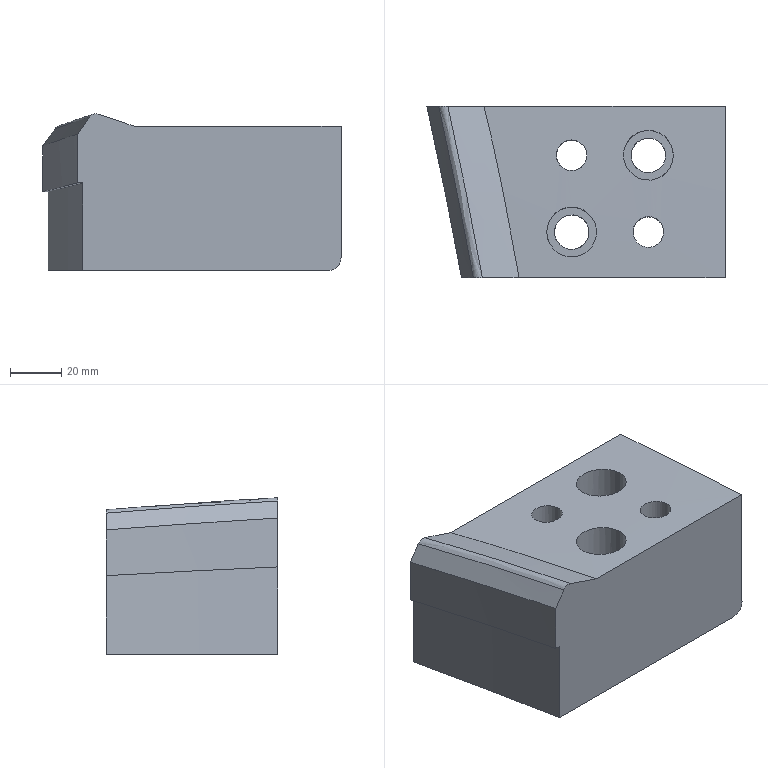Part | NX | features MAIN_BODY 2 | 1 solid | 22 faces | box 116.607 x 67 x 61.287 mm | volume 354263 mm3 | spline 9 | cylinder 7 | plane 6 | commonest cylinder face diameters 12 x2 13.5 x2 19.5 x2 10 x1
STEP:
#1=CARTESIAN_POINT('',(875.592,391.799,-36.703));
#2=VERTEX_POINT('',#1);
#3=CARTESIAN_POINT('',(875.621,399.722,-37.284));
#4=CARTESIAN_POINT('',(874.575,391.522,-36.682));
#5=CARTESIAN_POINT('',(879.631,384.982,-36.205));
#6=CARTESIAN_POINT('',(887.838,383.931,-36.131));
#7=CARTESIAN_POINT('',(894.382,388.999,-36.496));
#8=CARTESIAN_POINT('',(895.422,397.191,-37.099));
#9=CARTESIAN_POINT('',(890.383,403.727,-37.578));
#10=CARTESIAN_POINT('',(882.165,404.789,-37.656));
#11=CARTESIAN_POINT('',(875.621,399.722,-37.284));
#12=CARTESIAN_POINT('',(874.575,391.522,-36.682));
#13=CARTESIAN_POINT('',(879.631,384.982,-36.205));
#14=B_SPLINE_CURVE_WITH_KNOTS('',3,(#3,#4,#5,#6,#7,#8,#9,#10,#11,#12,#13),.UNSPECIFIED.,.T.,.F.,(1,1,1,1,1,1,1,1,1,1,1,1,1,1,1),(-0.02289,-0.01526,-0.00763,0.,0.00763,0.01526,0.02289,0.03052,0.03815,0.04578,0.05341,0.06104,0.06867,0.0763,0.08393),.UNSPECIFIED.);
#15=EDGE_CURVE('',#2,#2,#14,.T.);
#16=ORIENTED_EDGE('',*,*,#15,.F.);
#17=EDGE_LOOP('',(#16));
#18=FACE_BOUND('',#17,.T.);
#19=CARTESIAN_POINT('',(883.489,358.552,-34.446));
#20=VERTEX_POINT('',#19);
#21=CARTESIAN_POINT('',(879.261,361.,-34.597));
#22=CARTESIAN_POINT('',(883.325,357.92,-34.407));
#23=CARTESIAN_POINT('',(888.373,358.629,-34.45));
#24=CARTESIAN_POINT('',(891.432,362.685,-34.703));
#25=CARTESIAN_POINT('',(890.737,367.72,-35.026));
#26=CARTESIAN_POINT('',(886.676,370.794,-35.229));
#27=CARTESIAN_POINT('',(881.635,370.093,-35.183));
#28=CARTESIAN_POINT('',(878.567,366.035,-34.917));
#29=CARTESIAN_POINT('',(879.261,361.,-34.597));
#30=CARTESIAN_POINT('',(883.325,357.92,-34.407));
#31=CARTESIAN_POINT('',(888.373,358.629,-34.45));
#32=B_SPLINE_CURVE_WITH_KNOTS('',3,(#21,#22,#23,#24,#25,#26,#27,#28,#29,#30,#31),.UNSPECIFIED.,.T.,.F.,(1,1,1,1,1,1,1,1,1,1,1,1,1,1,1),(-0.01408,-0.009388,-0.004694,0.,0.004694,0.009388,0.01408,0.01878,0.02347,0.02816,0.03286,0.03755,0.04225,0.04694,0.05163),.UNSPECIFIED.);
#33=EDGE_CURVE('',#20,#20,#32,.T.);
#34=ORIENTED_EDGE('',*,*,#33,.F.);
#35=EDGE_LOOP('',(#34));
#36=FACE_BOUND('',#35,.T.);
#37=CARTESIAN_POINT('',(854.401,388.388,-36.453));
#38=VERTEX_POINT('',#37);
#39=CARTESIAN_POINT('',(849.844,390.159,-36.582));
#40=CARTESIAN_POINT('',(854.336,387.739,-36.405));
#41=CARTESIAN_POINT('',(859.216,389.217,-36.513));
#42=CARTESIAN_POINT('',(861.612,393.692,-36.842));
#43=CARTESIAN_POINT('',(860.154,398.56,-37.199));
#44=CARTESIAN_POINT('',(855.666,400.976,-37.376));
#45=CARTESIAN_POINT('',(850.791,399.506,-37.268));
#46=CARTESIAN_POINT('',(848.387,395.026,-36.939));
#47=CARTESIAN_POINT('',(849.844,390.159,-36.582));
#48=CARTESIAN_POINT('',(854.336,387.739,-36.405));
#49=CARTESIAN_POINT('',(859.216,389.217,-36.513));
#50=B_SPLINE_CURVE_WITH_KNOTS('',3,(#39,#40,#41,#42,#43,#44,#45,#46,#47,#48,#49),.UNSPECIFIED.,.T.,.F.,(1,1,1,1,1,1,1,1,1,1,1,1,1,1,1),(-0.01409,-0.009391,-0.004696,0.,0.004696,0.009391,0.01409,0.01878,0.02348,0.02817,0.03287,0.03756,0.04226,0.04696,0.05165),.UNSPECIFIED.);
#51=EDGE_CURVE('',#38,#38,#50,.T.);
#52=ORIENTED_EDGE('',*,*,#51,.F.);
#53=EDGE_LOOP('',(#52));
#54=FACE_BOUND('',#53,.T.);
#55=CARTESIAN_POINT('',(858.083,355.109,-34.235));
#56=VERTEX_POINT('',#55);
#57=CARTESIAN_POINT('',(850.147,354.7,-34.209));
#58=CARTESIAN_POINT('',(858.421,354.104,-34.174));
#59=CARTESIAN_POINT('',(864.664,359.534,-34.503));
#60=CARTESIAN_POINT('',(865.251,367.759,-35.026));
#61=CARTESIAN_POINT('',(859.849,374.018,-35.444));
#62=CARTESIAN_POINT('',(851.583,374.61,-35.485));
#63=CARTESIAN_POINT('',(845.343,369.198,-35.121));
#64=CARTESIAN_POINT('',(844.745,360.963,-34.592));
#65=CARTESIAN_POINT('',(850.147,354.7,-34.209));
#66=CARTESIAN_POINT('',(858.421,354.104,-34.174));
#67=CARTESIAN_POINT('',(864.664,359.534,-34.503));
#68=B_SPLINE_CURVE_WITH_KNOTS('',3,(#57,#58,#59,#60,#61,#62,#63,#64,#65,#66,#67),.UNSPECIFIED.,.T.,.F.,(1,1,1,1,1,1,1,1,1,1,1,1,1,1,1),(-0.02288,-0.01526,-0.007628,0.,0.007628,0.01526,0.02288,0.03051,0.03814,0.04577,0.05339,0.06102,0.06865,0.07628,0.0839),.UNSPECIFIED.);
#69=EDGE_CURVE('',#56,#56,#68,.T.);
#70=ORIENTED_EDGE('',*,*,#69,.F.);
#71=EDGE_LOOP('',(#70));
#72=FACE_BOUND('',#71,.T.);
#73=CARTESIAN_POINT('',(915.,346.533,-33.724));
#74=VERTEX_POINT('',#73);
#75=CARTESIAN_POINT('',(834.457,346.533,-33.724));
#76=VERTEX_POINT('',#75);
#77=CARTESIAN_POINT('',(873.245,346.533,-33.724));
#78=DIRECTION('',(-1.,0.000000011,-0.000000341));
#79=VECTOR('',#78,1000.);
#80=LINE('',#77,#79);
#81=EDGE_CURVE('',#74,#76,#80,.T.);
#82=ORIENTED_EDGE('',*,*,#81,.F.);
#83=CARTESIAN_POINT('',(915.,413.533,-38.297));
#84=VERTEX_POINT('',#83);
#85=CARTESIAN_POINT('',(915.,413.533,-38.297));
#86=CARTESIAN_POINT('',(915.,402.37,-37.478));
#87=CARTESIAN_POINT('',(915.,380.048,-35.784));
#88=CARTESIAN_POINT('',(915.,357.706,-34.385));
#89=CARTESIAN_POINT('',(915.,346.533,-33.724));
#90=B_SPLINE_CURVE_WITH_KNOTS('',3,(#85,#86,#87,#88,#89),.UNSPECIFIED.,.F.,.F.,(4,1,4),(0.271,0.3046,0.3382),.UNSPECIFIED.);
#91=EDGE_CURVE('',#84,#74,#90,.T.);
#92=ORIENTED_EDGE('',*,*,#91,.F.);
#93=CARTESIAN_POINT('',(820.678,413.533,-38.297));
#94=VERTEX_POINT('',#93);
#95=CARTESIAN_POINT('',(866.342,413.533,-38.297));
#96=DIRECTION('',(-1.,0.000000011,-0.000000341));
#97=VECTOR('',#96,1000.);
#98=LINE('',#95,#97);
#99=EDGE_CURVE('',#84,#94,#98,.T.);
#100=ORIENTED_EDGE('',*,*,#99,.T.);
#101=CARTESIAN_POINT('',(820.678,413.533,-38.297));
#102=CARTESIAN_POINT('',(822.089,408.009,-37.892));
#103=CARTESIAN_POINT('',(824.735,396.922,-37.08));
#104=CARTESIAN_POINT('',(829.299,374.584,-35.434));
#105=CARTESIAN_POINT('',(832.519,357.777,-34.389));
#106=CARTESIAN_POINT('',(834.457,346.533,-33.724));
#107=B_SPLINE_CURVE_WITH_KNOTS('',3,(#101,#102,#103,#104,#105,#106),.UNSPECIFIED.,.F.,.F.,(4,1,1,4),(0.,0.01714,0.03428,0.06856),.UNSPECIFIED.);
#108=EDGE_CURVE('',#94,#76,#107,.T.);
#109=ORIENTED_EDGE('',*,*,#108,.T.);
#110=EDGE_LOOP('',(#82,#92,#100,#109));
#111=FACE_BOUND('',#110,.T.);
#112=CARTESIAN_POINT('',(929.074,346.533,-33.724));
#113=CARTESIAN_POINT('',(833.62,346.533,-33.724));
#114=CARTESIAN_POINT('',(927.029,357.74,-34.387));
#115=CARTESIAN_POINT('',(831.575,357.74,-34.387));
#116=CARTESIAN_POINT('',(922.77,380.157,-35.792));
#117=CARTESIAN_POINT('',(827.316,380.157,-35.792));
#118=CARTESIAN_POINT('',(917.93,402.399,-37.48));
#119=CARTESIAN_POINT('',(822.476,402.399,-37.48));
#120=CARTESIAN_POINT('',(915.566,413.533,-38.297));
#121=CARTESIAN_POINT('',(820.112,413.533,-38.297));
#122=B_SPLINE_SURFACE_WITH_KNOTS('',3,1,((#112,#113),(#114,#115),(#116,#117),(#118,#119),(#120,#121)),.SURF_OF_LINEAR_EXTRUSION.,.F.,.F.,.F.,(4,1,4),(2,2),(-0.1003,0.757,1.614),(0.,1.),.UNSPECIFIED.);
#123=ADVANCED_FACE('',(#18,#36,#54,#72,#111),#122,.T.);
#124=CARTESIAN_POINT('',(798.461,413.533,-41.305));
#125=VERTEX_POINT('',#124);
#126=CARTESIAN_POINT('',(798.393,413.533,-41.305));
#127=VERTEX_POINT('',#126);
#128=CARTESIAN_POINT('',(871.04,413.533,-41.305));
#129=DIRECTION('',(-1.,0.000000011,-0.000000341));
#130=VECTOR('',#129,1000.);
#131=LINE('',#128,#130);
#132=EDGE_CURVE('',#125,#127,#131,.T.);
#133=ORIENTED_EDGE('',*,*,#132,.T.);
#134=CARTESIAN_POINT('',(804.549,384.498,-39.18));
#135=VERTEX_POINT('',#134);
#136=CARTESIAN_POINT('',(798.393,413.533,-41.305));
#137=CARTESIAN_POINT('',(800.448,403.855,-40.595));
#138=CARTESIAN_POINT('',(802.53,394.184,-39.872));
#139=CARTESIAN_POINT('',(804.549,384.498,-39.18));
#140=B_SPLINE_CURVE_WITH_KNOTS('',3,(#136,#137,#138,#139),.UNSPECIFIED.,.F.,.F.,(4,4),(0.,0.02976),.UNSPECIFIED.);
#141=EDGE_CURVE('',#127,#135,#140,.T.);
#142=ORIENTED_EDGE('',*,*,#141,.T.);
#143=CARTESIAN_POINT('',(798.461,413.533,-41.305));
#144=CARTESIAN_POINT('',(800.491,403.855,-40.595));
#145=CARTESIAN_POINT('',(802.531,394.18,-39.872));
#146=CARTESIAN_POINT('',(804.549,384.498,-39.18));
#147=B_SPLINE_CURVE_WITH_KNOTS('',3,(#143,#144,#145,#146),.UNSPECIFIED.,.F.,.F.,(4,4),(0.,0.02974),.UNSPECIFIED.);
#148=EDGE_CURVE('',#125,#135,#147,.T.);
#149=ORIENTED_EDGE('',*,*,#148,.F.);
#150=EDGE_LOOP('',(#133,#142,#149));
#151=FACE_BOUND('',#150,.T.);
#152=CARTESIAN_POINT('',(804.654,384.324,-39.167));
#153=CARTESIAN_POINT('',(804.586,384.324,-39.167));
#154=CARTESIAN_POINT('',(802.624,394.068,-39.863));
#155=CARTESIAN_POINT('',(802.556,394.068,-39.863));
#156=CARTESIAN_POINT('',(800.529,403.797,-40.591));
#157=CARTESIAN_POINT('',(800.461,403.797,-40.591));
#158=CARTESIAN_POINT('',(798.461,413.533,-41.305));
#159=CARTESIAN_POINT('',(798.393,413.533,-41.305));
#160=B_SPLINE_SURFACE_WITH_KNOTS('',3,1,((#152,#153),(#154,#155),(#156,#157),(#158,#159)),.SURF_OF_LINEAR_EXTRUSION.,.F.,.F.,.F.,(4,4),(2,2),(0.8703,1.62),(0.,1.),.PIECEWISE_BEZIER_KNOTS.);
#161=ADVANCED_FACE('',(#151),#160,.T.);
#162=CARTESIAN_POINT('',(885.,387.608,-90.));
#163=VERTEX_POINT('',#162);
#164=CARTESIAN_POINT('',(885.,394.358,-90.));
#165=DIRECTION('',(0.000000341,-0.00000017,-1.));
#166=DIRECTION('',(-0.000000011,-1.,0.00000017));
#167=AXIS2_PLACEMENT_3D('',#164,#165,#166);
#168=CIRCLE('',#167,6.75);
#169=EDGE_CURVE('',#163,#163,#168,.T.);
#170=ORIENTED_EDGE('',*,*,#169,.F.);
#171=EDGE_LOOP('',(#170));
#172=FACE_BOUND('',#171,.T.);
#173=CARTESIAN_POINT('',(885.,358.358,-90.));
#174=VERTEX_POINT('',#173);
#175=CARTESIAN_POINT('',(885.,364.358,-90.));
#176=DIRECTION('',(0.000000341,-0.00000017,-1.));
#177=DIRECTION('',(-0.000000011,-1.,0.00000017));
#178=AXIS2_PLACEMENT_3D('',#175,#176,#177);
#179=CIRCLE('',#178,6.);
#180=EDGE_CURVE('',#174,#174,#179,.T.);
#181=ORIENTED_EDGE('',*,*,#180,.F.);
#182=EDGE_LOOP('',(#181));
#183=FACE_BOUND('',#182,.T.);
#184=CARTESIAN_POINT('',(855.,357.608,-90.));
#185=VERTEX_POINT('',#184);
#186=CARTESIAN_POINT('',(855.,364.358,-90.));
#187=DIRECTION('',(0.000000341,-0.00000017,-1.));
#188=DIRECTION('',(-0.000000011,-1.,0.00000017));
#189=AXIS2_PLACEMENT_3D('',#186,#187,#188);
#190=CIRCLE('',#189,6.75);
#191=EDGE_CURVE('',#185,#185,#190,.T.);
#192=ORIENTED_EDGE('',*,*,#191,.F.);
#193=EDGE_LOOP('',(#192));
#194=FACE_BOUND('',#193,.T.);
#195=CARTESIAN_POINT('',(855.,388.358,-90.));
#196=VERTEX_POINT('',#195);
#197=CARTESIAN_POINT('',(855.,394.358,-90.));
#198=DIRECTION('',(0.000000341,-0.00000017,-1.));
#199=DIRECTION('',(-0.000000011,-1.,0.00000017));
#200=AXIS2_PLACEMENT_3D('',#197,#198,#199);
#201=CIRCLE('',#200,6.);
#202=EDGE_CURVE('',#196,#196,#201,.T.);
#203=ORIENTED_EDGE('',*,*,#202,.F.);
#204=EDGE_LOOP('',(#203));
#205=FACE_BOUND('',#204,.T.);
#206=CARTESIAN_POINT('',(910.,346.533,-90.));
#207=VERTEX_POINT('',#206);
#208=CARTESIAN_POINT('',(813.948,346.533,-90.));
#209=VERTEX_POINT('',#208);
#210=CARTESIAN_POINT('',(830.,346.533,-90.));
#211=DIRECTION('',(-1.,0.000000011,-0.000000341));
#212=VECTOR('',#211,1000.);
#213=LINE('',#210,#212);
#214=EDGE_CURVE('',#207,#209,#213,.T.);
#215=ORIENTED_EDGE('',*,*,#214,.T.);
#216=CARTESIAN_POINT('',(800.438,413.533,-90.));
#217=VERTEX_POINT('',#216);
#218=CARTESIAN_POINT('',(800.438,413.533,-90.));
#219=CARTESIAN_POINT('',(802.804,402.389,-90.));
#220=CARTESIAN_POINT('',(807.649,380.124,-90.));
#221=CARTESIAN_POINT('',(811.904,357.74,-90.));
#222=CARTESIAN_POINT('',(813.948,346.533,-90.));
#223=B_SPLINE_CURVE_WITH_KNOTS('',3,(#218,#219,#220,#221,#222),.UNSPECIFIED.,.F.,.F.,(4,1,4),(0.,0.03418,0.06835),.UNSPECIFIED.);
#224=EDGE_CURVE('',#217,#209,#223,.T.);
#225=ORIENTED_EDGE('',*,*,#224,.F.);
#226=CARTESIAN_POINT('',(910.,413.533,-90.));
#227=VERTEX_POINT('',#226);
#228=CARTESIAN_POINT('',(830.,413.533,-90.));
#229=DIRECTION('',(-1.,0.000000011,-0.000000341));
#230=VECTOR('',#229,1000.);
#231=LINE('',#228,#230);
#232=EDGE_CURVE('',#227,#217,#231,.T.);
#233=ORIENTED_EDGE('',*,*,#232,.F.);
#234=CARTESIAN_POINT('',(910.,413.533,-90.));
#235=DIRECTION('',(0.000000011,1.,-0.00000017));
#236=VECTOR('',#235,1000.);
#237=LINE('',#234,#236);
#238=EDGE_CURVE('',#207,#227,#237,.T.);
#239=ORIENTED_EDGE('',*,*,#238,.F.);
#240=EDGE_LOOP('',(#215,#225,#233,#239));
#241=FACE_BOUND('',#240,.T.);
#242=CARTESIAN_POINT('',(830.,1053.533,-90.));
#243=DIRECTION('',(0.000000341,-0.00000017,-1.));
#244=DIRECTION('',(0.000000011,1.,-0.00000017));
#245=AXIS2_PLACEMENT_3D('',#242,#243,#244);
#246=PLANE('',#245);
#247=ADVANCED_FACE('',(#172,#183,#194,#205,#241),#246,.T.);
#248=CARTESIAN_POINT('',(806.592,413.533,-33.58));
#249=VERTEX_POINT('',#248);
#250=CARTESIAN_POINT('',(806.592,413.533,-33.58));
#251=CARTESIAN_POINT('',(811.287,413.533,-35.152));
#252=CARTESIAN_POINT('',(815.982,413.533,-36.725));
#253=CARTESIAN_POINT('',(820.678,413.533,-38.297));
#254=B_SPLINE_CURVE_WITH_KNOTS('',3,(#250,#251,#252,#253),.UNSPECIFIED.,.F.,.F.,(4,4),(0.002341,0.0172),.UNSPECIFIED.);
#255=EDGE_CURVE('',#249,#94,#254,.T.);
#256=ORIENTED_EDGE('',*,*,#255,.T.);
#257=ORIENTED_EDGE('',*,*,#99,.F.);
#258=CARTESIAN_POINT('',(915.,413.533,-85.));
#259=VERTEX_POINT('',#258);
#260=CARTESIAN_POINT('',(915.,413.533,-90.));
#261=DIRECTION('',(0.000000341,-0.00000017,-1.));
#262=VECTOR('',#261,1000.);
#263=LINE('',#260,#262);
#264=EDGE_CURVE('',#259,#84,#263,.F.);
#265=ORIENTED_EDGE('',*,*,#264,.F.);
#266=CARTESIAN_POINT('',(910.,413.533,-85.));
#267=DIRECTION('',(-0.000000011,-1.,0.00000017));
#268=DIRECTION('',(-0.000000341,0.00000017,1.));
#269=AXIS2_PLACEMENT_3D('',#266,#267,#268);
#270=CIRCLE('',#269,5.);
#271=EDGE_CURVE('',#227,#259,#270,.T.);
#272=ORIENTED_EDGE('',*,*,#271,.F.);
#273=ORIENTED_EDGE('',*,*,#232,.T.);
#274=CARTESIAN_POINT('',(800.438,413.533,-59.211));
#275=VERTEX_POINT('',#274);
#276=CARTESIAN_POINT('',(800.438,413.533,-59.211));
#277=CARTESIAN_POINT('',(800.438,413.533,-69.474));
#278=CARTESIAN_POINT('',(800.438,413.533,-79.737));
#279=CARTESIAN_POINT('',(800.438,413.533,-90.));
#280=B_SPLINE_CURVE_WITH_KNOTS('',3,(#276,#277,#278,#279),.UNSPECIFIED.,.F.,.F.,(4,4),(0.,0.03079),.UNSPECIFIED.);
#281=EDGE_CURVE('',#275,#217,#280,.T.);
#282=ORIENTED_EDGE('',*,*,#281,.F.);
#283=CARTESIAN_POINT('',(798.393,413.533,-59.226));
#284=VERTEX_POINT('',#283);
#285=CARTESIAN_POINT('',(800.438,413.533,-59.211));
#286=CARTESIAN_POINT('',(799.756,413.533,-59.216));
#287=CARTESIAN_POINT('',(799.075,413.533,-59.221));
#288=CARTESIAN_POINT('',(798.393,413.533,-59.226));
#289=B_SPLINE_CURVE_WITH_KNOTS('',3,(#285,#286,#287,#288),.UNSPECIFIED.,.F.,.F.,(4,4),(0.003448,0.005492),.UNSPECIFIED.);
#290=EDGE_CURVE('',#275,#284,#289,.T.);
#291=ORIENTED_EDGE('',*,*,#290,.T.);
#292=CARTESIAN_POINT('',(798.393,413.533,-41.305));
#293=CARTESIAN_POINT('',(798.393,413.533,-47.279));
#294=CARTESIAN_POINT('',(798.393,413.533,-53.252));
#295=CARTESIAN_POINT('',(798.393,413.533,-59.226));
#296=B_SPLINE_CURVE_WITH_KNOTS('',3,(#292,#293,#294,#295),.UNSPECIFIED.,.F.,.F.,(4,4),(0.,0.01792),.UNSPECIFIED.);
#297=EDGE_CURVE('',#127,#284,#296,.T.);
#298=ORIENTED_EDGE('',*,*,#297,.F.);
#299=ORIENTED_EDGE('',*,*,#132,.F.);
#300=CARTESIAN_POINT('',(803.028,413.533,-34.762));
#301=VERTEX_POINT('',#300);
#302=CARTESIAN_POINT('',(803.028,413.533,-34.762));
#303=CARTESIAN_POINT('',(801.506,413.533,-36.943));
#304=CARTESIAN_POINT('',(799.983,413.533,-39.124));
#305=CARTESIAN_POINT('',(798.461,413.533,-41.305));
#306=B_SPLINE_CURVE_WITH_KNOTS('',3,(#302,#303,#304,#305),.UNSPECIFIED.,.F.,.F.,(4,4),(0.002349,0.01033),.UNSPECIFIED.);
#307=EDGE_CURVE('',#301,#125,#306,.T.);
#308=ORIENTED_EDGE('',*,*,#307,.F.);
#309=CARTESIAN_POINT('',(806.592,413.533,-33.58));
#310=CARTESIAN_POINT('',(805.308,413.533,-33.15));
#311=CARTESIAN_POINT('',(803.802,413.533,-33.652));
#312=CARTESIAN_POINT('',(803.028,413.533,-34.762));
#313=B_SPLINE_CURVE_WITH_KNOTS('',3,(#309,#310,#311,#312),.UNSPECIFIED.,.F.,.F.,(4,4),(0.,0.004002),.UNSPECIFIED.);
#314=EDGE_CURVE('',#249,#301,#313,.T.);
#315=ORIENTED_EDGE('',*,*,#314,.F.);
#316=EDGE_LOOP('',(#256,#257,#265,#272,#273,#282,#291,#298,#299,#308,#315));
#317=FACE_BOUND('',#316,.T.);
#318=CARTESIAN_POINT('',(890.,413.533,-90.));
#319=DIRECTION('',(0.000000011,1.,-0.00000017));
#320=DIRECTION('',(-0.000000341,0.00000017,1.));
#321=AXIS2_PLACEMENT_3D('',#318,#319,#320);
#322=PLANE('',#321);
#323=ADVANCED_FACE('',(#317),#322,.T.);
#324=ORIENTED_EDGE('',*,*,#141,.F.);
#325=ORIENTED_EDGE('',*,*,#297,.T.);
#326=CARTESIAN_POINT('',(811.915,346.533,-55.81));
#327=VERTEX_POINT('',#326);
#328=CARTESIAN_POINT('',(798.393,413.533,-59.226));
#329=CARTESIAN_POINT('',(800.759,402.391,-58.614));
#330=CARTESIAN_POINT('',(805.603,380.131,-57.36));
#331=CARTESIAN_POINT('',(809.87,357.743,-56.321));
#332=CARTESIAN_POINT('',(811.915,346.533,-55.81));
#333=B_SPLINE_CURVE_WITH_KNOTS('',3,(#328,#329,#330,#331,#332),.UNSPECIFIED.,.F.,.F.,(4,1,4),(0.,0.03422,0.06844),.UNSPECIFIED.);
#334=EDGE_CURVE('',#284,#327,#333,.T.);
#335=ORIENTED_EDGE('',*,*,#334,.T.);
#336=CARTESIAN_POINT('',(811.915,346.533,-36.73));
#337=VERTEX_POINT('',#336);
#338=CARTESIAN_POINT('',(811.915,346.533,-36.73));
#339=CARTESIAN_POINT('',(811.915,346.533,-43.09));
#340=CARTESIAN_POINT('',(811.915,346.533,-49.45));
#341=CARTESIAN_POINT('',(811.915,346.533,-55.81));
#342=B_SPLINE_CURVE_WITH_KNOTS('',3,(#338,#339,#340,#341),.UNSPECIFIED.,.F.,.F.,(4,4),(0.,0.01908),.UNSPECIFIED.);
#343=EDGE_CURVE('',#337,#327,#342,.T.);
#344=ORIENTED_EDGE('',*,*,#343,.F.);
#345=CARTESIAN_POINT('',(810.326,355.197,-37.246));
#346=VERTEX_POINT('',#345);
#347=CARTESIAN_POINT('',(810.326,355.197,-37.246));
#348=CARTESIAN_POINT('',(810.863,352.311,-37.07));
#349=CARTESIAN_POINT('',(811.388,349.422,-36.9));
#350=CARTESIAN_POINT('',(811.915,346.533,-36.73));
#351=B_SPLINE_CURVE_WITH_KNOTS('',3,(#347,#348,#349,#350),.UNSPECIFIED.,.F.,.F.,(4,4),(0.05968,0.06851),.UNSPECIFIED.);
#352=EDGE_CURVE('',#346,#337,#351,.T.);
#353=ORIENTED_EDGE('',*,*,#352,.F.);
#354=CARTESIAN_POINT('',(804.549,384.498,-39.18));
#355=CARTESIAN_POINT('',(806.58,374.756,-38.484));
#356=CARTESIAN_POINT('',(808.504,364.988,-37.841));
#357=CARTESIAN_POINT('',(810.326,355.197,-37.246));
#358=B_SPLINE_CURVE_WITH_KNOTS('',3,(#354,#355,#356,#357),.UNSPECIFIED.,.F.,.F.,(4,4),(0.02976,0.05969),.UNSPECIFIED.);
#359=EDGE_CURVE('',#135,#346,#358,.T.);
#360=ORIENTED_EDGE('',*,*,#359,.F.);
#361=EDGE_LOOP('',(#324,#325,#335,#344,#353,#360));
#362=FACE_BOUND('',#361,.T.);
#363=CARTESIAN_POINT('',(811.989,346.129,-55.901));
#364=CARTESIAN_POINT('',(811.989,346.129,-36.706));
#365=CARTESIAN_POINT('',(809.919,357.478,-56.572));
#366=CARTESIAN_POINT('',(809.919,357.478,-37.376));
#367=CARTESIAN_POINT('',(805.606,380.136,-57.992));
#368=CARTESIAN_POINT('',(805.606,380.136,-38.797));
#369=CARTESIAN_POINT('',(800.702,402.659,-59.703));
#370=CARTESIAN_POINT('',(800.702,402.659,-40.507));
#371=CARTESIAN_POINT('',(798.308,413.934,-60.53));
#372=CARTESIAN_POINT('',(798.308,413.934,-41.335));
#373=B_SPLINE_SURFACE_WITH_KNOTS('',3,1,((#363,#364),(#365,#366),(#367,#368),(#369,#370),(#371,#372)),.SURF_OF_LINEAR_EXTRUSION.,.F.,.F.,.F.,(4,1,4),(2,2),(-0.1061,0.7621,1.63),(0.,1.),.UNSPECIFIED.);
#374=ADVANCED_FACE('',(#362),#373,.F.);
#375=ORIENTED_EDGE('',*,*,#264,.T.);
#376=ORIENTED_EDGE('',*,*,#91,.T.);
#377=CARTESIAN_POINT('',(915.,346.533,-85.));
#378=VERTEX_POINT('',#377);
#379=CARTESIAN_POINT('',(915.,346.533,-90.));
#380=DIRECTION('',(0.000000341,-0.00000017,-1.));
#381=VECTOR('',#380,1000.);
#382=LINE('',#379,#381);
#383=EDGE_CURVE('',#378,#74,#382,.F.);
#384=ORIENTED_EDGE('',*,*,#383,.F.);
#385=CARTESIAN_POINT('',(915.,346.533,-85.));
#386=DIRECTION('',(-0.000000011,-1.,0.00000017));
#387=VECTOR('',#386,1000.);
#388=LINE('',#385,#387);
#389=EDGE_CURVE('',#259,#378,#388,.T.);
#390=ORIENTED_EDGE('',*,*,#389,.F.);
#391=EDGE_LOOP('',(#375,#376,#384,#390));
#392=FACE_BOUND('',#391,.T.);
#393=CARTESIAN_POINT('',(915.,734.25,-90.));
#394=DIRECTION('',(1.,-0.000000011,0.000000341));
#395=DIRECTION('',(0.000000341,-0.00000017,-1.));
#396=AXIS2_PLACEMENT_3D('',#393,#394,#395);
#397=PLANE('',#396);
#398=ADVANCED_FACE('',(#392),#397,.T.);
#399=ORIENTED_EDGE('',*,*,#352,.T.);
#400=CARTESIAN_POINT('',(811.931,346.533,-36.73));
#401=VERTEX_POINT('',#400);
#402=CARTESIAN_POINT('',(875.23,346.533,-36.73));
#403=DIRECTION('',(-1.,0.000000011,-0.000000341));
#404=VECTOR('',#403,1000.);
#405=LINE('',#402,#404);
#406=EDGE_CURVE('',#401,#337,#405,.T.);
#407=ORIENTED_EDGE('',*,*,#406,.F.);
#408=CARTESIAN_POINT('',(810.326,355.197,-37.246));
#409=CARTESIAN_POINT('',(810.863,352.31,-37.07));
#410=CARTESIAN_POINT('',(811.397,349.421,-36.9));
#411=CARTESIAN_POINT('',(811.931,346.533,-36.73));
#412=B_SPLINE_CURVE_WITH_KNOTS('',3,(#408,#409,#410,#411),.UNSPECIFIED.,.F.,.F.,(4,4),(0.05967,0.0685),.UNSPECIFIED.);
#413=EDGE_CURVE('',#346,#401,#412,.T.);
#414=ORIENTED_EDGE('',*,*,#413,.F.);
#415=EDGE_LOOP('',(#399,#407,#414));
#416=FACE_BOUND('',#415,.T.);
#417=CARTESIAN_POINT('',(811.931,346.533,-36.73));
#418=CARTESIAN_POINT('',(811.915,346.533,-36.73));
#419=CARTESIAN_POINT('',(811.401,349.439,-36.901));
#420=CARTESIAN_POINT('',(811.385,349.439,-36.901));
#421=CARTESIAN_POINT('',(810.872,352.345,-37.072));
#422=CARTESIAN_POINT('',(810.857,352.345,-37.072));
#423=CARTESIAN_POINT('',(810.332,355.249,-37.249));
#424=CARTESIAN_POINT('',(810.316,355.249,-37.249));
#425=B_SPLINE_SURFACE_WITH_KNOTS('',3,1,((#417,#418),(#419,#420),(#421,#422),(#423,#424)),.SURF_OF_LINEAR_EXTRUSION.,.F.,.F.,.F.,(4,4),(2,2),(-0.09577,0.1265),(0.,1.),.PIECEWISE_BEZIER_KNOTS.);
#426=ADVANCED_FACE('',(#416),#425,.T.);
#427=CARTESIAN_POINT('',(816.542,346.533,-30.039));
#428=VERTEX_POINT('',#427);
#429=CARTESIAN_POINT('',(811.931,346.533,-36.73));
#430=CARTESIAN_POINT('',(813.468,346.533,-34.5));
#431=CARTESIAN_POINT('',(815.005,346.533,-32.27));
#432=CARTESIAN_POINT('',(816.542,346.533,-30.039));
#433=B_SPLINE_CURVE_WITH_KNOTS('',3,(#429,#430,#431,#432),.UNSPECIFIED.,.F.,.F.,(4,4),(0.00002698,0.008152),.UNSPECIFIED.);
#434=EDGE_CURVE('',#401,#428,#433,.T.);
#435=ORIENTED_EDGE('',*,*,#434,.F.);
#436=ORIENTED_EDGE('',*,*,#406,.T.);
#437=ORIENTED_EDGE('',*,*,#343,.T.);
#438=CARTESIAN_POINT('',(813.948,346.533,-55.8));
#439=VERTEX_POINT('',#438);
#440=CARTESIAN_POINT('',(811.915,346.533,-55.81));
#441=CARTESIAN_POINT('',(812.593,346.533,-55.807));
#442=CARTESIAN_POINT('',(813.271,346.533,-55.803));
#443=CARTESIAN_POINT('',(813.948,346.533,-55.8));
#444=B_SPLINE_CURVE_WITH_KNOTS('',3,(#440,#441,#442,#443),.UNSPECIFIED.,.F.,.F.,(4,4),(0.001632,0.003665),.UNSPECIFIED.);
#445=EDGE_CURVE('',#327,#439,#444,.T.);
#446=ORIENTED_EDGE('',*,*,#445,.T.);
#447=CARTESIAN_POINT('',(813.948,346.533,-55.8));
#448=CARTESIAN_POINT('',(813.948,346.533,-67.2));
#449=CARTESIAN_POINT('',(813.948,346.533,-78.6));
#450=CARTESIAN_POINT('',(813.948,346.533,-90.));
#451=B_SPLINE_CURVE_WITH_KNOTS('',3,(#447,#448,#449,#450),.UNSPECIFIED.,.F.,.F.,(4,4),(0.,0.0342),.UNSPECIFIED.);
#452=EDGE_CURVE('',#439,#209,#451,.T.);
#453=ORIENTED_EDGE('',*,*,#452,.T.);
#454=ORIENTED_EDGE('',*,*,#214,.F.);
#455=CARTESIAN_POINT('',(910.,346.533,-85.));
#456=DIRECTION('',(-0.000000011,-1.,0.00000017));
#457=DIRECTION('',(-0.000000341,0.00000017,1.));
#458=AXIS2_PLACEMENT_3D('',#455,#456,#457);
#459=CIRCLE('',#458,5.);
#460=EDGE_CURVE('',#378,#207,#459,.F.);
#461=ORIENTED_EDGE('',*,*,#460,.F.);
#462=ORIENTED_EDGE('',*,*,#383,.T.);
#463=ORIENTED_EDGE('',*,*,#81,.T.);
#464=CARTESIAN_POINT('',(820.074,346.533,-28.867));
#465=VERTEX_POINT('',#464);
#466=CARTESIAN_POINT('',(820.074,346.533,-28.867));
#467=CARTESIAN_POINT('',(824.868,346.533,-30.486));
#468=CARTESIAN_POINT('',(829.662,346.533,-32.105));
#469=CARTESIAN_POINT('',(834.457,346.533,-33.724));
#470=B_SPLINE_CURVE_WITH_KNOTS('',3,(#466,#467,#468,#469),.UNSPECIFIED.,.F.,.F.,(4,4),(0.002332,0.01751),.UNSPECIFIED.);
#471=EDGE_CURVE('',#465,#76,#470,.T.);
#472=ORIENTED_EDGE('',*,*,#471,.F.);
#473=CARTESIAN_POINT('',(816.542,346.533,-30.039));
#474=CARTESIAN_POINT('',(817.304,346.533,-28.933));
#475=CARTESIAN_POINT('',(818.801,346.533,-28.437));
#476=CARTESIAN_POINT('',(820.074,346.533,-28.867));
#477=B_SPLINE_CURVE_WITH_KNOTS('',3,(#473,#474,#475,#476),.UNSPECIFIED.,.F.,.F.,(4,4),(0.,0.003971),.UNSPECIFIED.);
#478=EDGE_CURVE('',#428,#465,#477,.T.);
#479=ORIENTED_EDGE('',*,*,#478,.F.);
#480=EDGE_LOOP('',(#435,#436,#437,#446,#453,#454,#461,#462,#463,#472,#479));
#481=FACE_BOUND('',#480,.T.);
#482=CARTESIAN_POINT('',(890.,346.533,-90.));
#483=DIRECTION('',(0.000000011,1.,-0.00000017));
#484=DIRECTION('',(-0.000000341,0.00000017,1.));
#485=AXIS2_PLACEMENT_3D('',#482,#483,#484);
#486=PLANE('',#485);
#487=ADVANCED_FACE('',(#481),#486,.F.);
#488=CARTESIAN_POINT('',(894.75,394.358,-80.));
#489=VERTEX_POINT('',#488);
#490=CARTESIAN_POINT('',(885.,394.358,-80.));
#491=DIRECTION('',(-0.000000341,0.00000017,1.));
#492=DIRECTION('',(1.,0.,0.000000341));
#493=AXIS2_PLACEMENT_3D('',#490,#491,#492);
#494=CIRCLE('',#493,9.75);
#495=EDGE_CURVE('',#489,#489,#494,.F.);
#496=ORIENTED_EDGE('',*,*,#495,.T.);
#497=EDGE_LOOP('',(#496));
#498=FACE_BOUND('',#497,.T.);
#499=ORIENTED_EDGE('',*,*,#15,.T.);
#500=EDGE_LOOP('',(#499));
#501=FACE_BOUND('',#500,.T.);
#502=CARTESIAN_POINT('',(885.,394.358,-70.));
#503=DIRECTION('',(-0.000000341,0.00000017,1.));
#504=DIRECTION('',(-0.000000011,-1.,0.00000017));
#505=AXIS2_PLACEMENT_3D('',#502,#503,#504);
#506=CYLINDRICAL_SURFACE('',#505,9.75);
#507=ADVANCED_FACE('',(#498,#501),#506,.F.);
#508=CARTESIAN_POINT('',(891.75,394.358,-80.));
#509=VERTEX_POINT('',#508);
#510=CARTESIAN_POINT('',(885.,394.358,-80.));
#511=DIRECTION('',(-0.000000341,0.00000017,1.));
#512=DIRECTION('',(1.,0.,0.000000341));
#513=AXIS2_PLACEMENT_3D('',#510,#511,#512);
#514=CIRCLE('',#513,6.75);
#515=EDGE_CURVE('',#509,#509,#514,.F.);
#516=ORIENTED_EDGE('',*,*,#515,.F.);
#517=EDGE_LOOP('',(#516));
#518=FACE_BOUND('',#517,.T.);
#519=ORIENTED_EDGE('',*,*,#169,.T.);
#520=EDGE_LOOP('',(#519));
#521=FACE_BOUND('',#520,.T.);
#522=CARTESIAN_POINT('',(885.,394.358,-90.));
#523=DIRECTION('',(-0.000000341,0.00000017,1.));
#524=DIRECTION('',(-0.000000011,-1.,0.00000017));
#525=AXIS2_PLACEMENT_3D('',#522,#523,#524);
#526=CYLINDRICAL_SURFACE('',#525,6.75);
#527=ADVANCED_FACE('',(#518,#521),#526,.F.);
#528=ORIENTED_EDGE('',*,*,#515,.T.);
#529=EDGE_LOOP('',(#528));
#530=FACE_BOUND('',#529,.T.);
#531=ORIENTED_EDGE('',*,*,#495,.F.);
#532=EDGE_LOOP('',(#531));
#533=FACE_BOUND('',#532,.T.);
#534=CARTESIAN_POINT('',(885.,394.358,-80.));
#535=DIRECTION('',(0.000000341,-0.00000017,-1.));
#536=DIRECTION('',(0.000000011,1.,-0.00000017));
#537=AXIS2_PLACEMENT_3D('',#534,#535,#536);
#538=PLANE('',#537);
#539=ADVANCED_FACE('',(#530,#533),#538,.F.);
#540=ORIENTED_EDGE('',*,*,#180,.T.);
#541=EDGE_LOOP('',(#540));
#542=FACE_BOUND('',#541,.T.);
#543=ORIENTED_EDGE('',*,*,#33,.T.);
#544=EDGE_LOOP('',(#543));
#545=FACE_BOUND('',#544,.T.);
#546=CARTESIAN_POINT('',(885.,364.358,-90.));
#547=DIRECTION('',(-0.000000341,0.00000017,1.));
#548=DIRECTION('',(-0.000000011,-1.,0.00000017));
#549=AXIS2_PLACEMENT_3D('',#546,#547,#548);
#550=CYLINDRICAL_SURFACE('',#549,6.);
#551=ADVANCED_FACE('',(#542,#545),#550,.F.);
#552=CARTESIAN_POINT('',(864.75,364.358,-80.));
#553=VERTEX_POINT('',#552);
#554=CARTESIAN_POINT('',(855.,364.358,-80.));
#555=DIRECTION('',(-0.000000341,0.00000017,1.));
#556=DIRECTION('',(1.,0.,0.000000341));
#557=AXIS2_PLACEMENT_3D('',#554,#555,#556);
#558=CIRCLE('',#557,9.75);
#559=EDGE_CURVE('',#553,#553,#558,.F.);
#560=ORIENTED_EDGE('',*,*,#559,.T.);
#561=EDGE_LOOP('',(#560));
#562=FACE_BOUND('',#561,.T.);
#563=ORIENTED_EDGE('',*,*,#69,.T.);
#564=EDGE_LOOP('',(#563));
#565=FACE_BOUND('',#564,.T.);
#566=CARTESIAN_POINT('',(855.,364.358,-70.));
#567=DIRECTION('',(-0.000000341,0.00000017,1.));
#568=DIRECTION('',(-0.000000011,-1.,0.00000017));
#569=AXIS2_PLACEMENT_3D('',#566,#567,#568);
#570=CYLINDRICAL_SURFACE('',#569,9.75);
#571=ADVANCED_FACE('',(#562,#565),#570,.F.);
#572=CARTESIAN_POINT('',(861.75,364.358,-80.));
#573=VERTEX_POINT('',#572);
#574=CARTESIAN_POINT('',(855.,364.358,-80.));
#575=DIRECTION('',(-0.000000341,0.00000017,1.));
#576=DIRECTION('',(1.,0.,0.000000341));
#577=AXIS2_PLACEMENT_3D('',#574,#575,#576);
#578=CIRCLE('',#577,6.75);
#579=EDGE_CURVE('',#573,#573,#578,.F.);
#580=ORIENTED_EDGE('',*,*,#579,.F.);
#581=EDGE_LOOP('',(#580));
#582=FACE_BOUND('',#581,.T.);
#583=ORIENTED_EDGE('',*,*,#191,.T.);
#584=EDGE_LOOP('',(#583));
#585=FACE_BOUND('',#584,.T.);
#586=CARTESIAN_POINT('',(855.,364.358,-90.));
#587=DIRECTION('',(-0.000000341,0.00000017,1.));
#588=DIRECTION('',(-0.000000011,-1.,0.00000017));
#589=AXIS2_PLACEMENT_3D('',#586,#587,#588);
#590=CYLINDRICAL_SURFACE('',#589,6.75);
#591=ADVANCED_FACE('',(#582,#585),#590,.F.);
#592=ORIENTED_EDGE('',*,*,#579,.T.);
#593=EDGE_LOOP('',(#592));
#594=FACE_BOUND('',#593,.T.);
#595=ORIENTED_EDGE('',*,*,#559,.F.);
#596=EDGE_LOOP('',(#595));
#597=FACE_BOUND('',#596,.T.);
#598=CARTESIAN_POINT('',(855.,364.358,-80.));
#599=DIRECTION('',(0.000000341,-0.00000017,-1.));
#600=DIRECTION('',(0.000000011,1.,-0.00000017));
#601=AXIS2_PLACEMENT_3D('',#598,#599,#600);
#602=PLANE('',#601);
#603=ADVANCED_FACE('',(#594,#597),#602,.F.);
#604=ORIENTED_EDGE('',*,*,#202,.T.);
#605=EDGE_LOOP('',(#604));
#606=FACE_BOUND('',#605,.T.);
#607=ORIENTED_EDGE('',*,*,#51,.T.);
#608=EDGE_LOOP('',(#607));
#609=FACE_BOUND('',#608,.T.);
#610=CARTESIAN_POINT('',(855.,394.358,-90.));
#611=DIRECTION('',(-0.000000341,0.00000017,1.));
#612=DIRECTION('',(-0.000000011,-1.,0.00000017));
#613=AXIS2_PLACEMENT_3D('',#610,#611,#612);
#614=CYLINDRICAL_SURFACE('',#613,6.);
#615=ADVANCED_FACE('',(#606,#609),#614,.F.);
#616=ORIENTED_EDGE('',*,*,#290,.F.);
#617=CARTESIAN_POINT('',(800.438,413.533,-59.211));
#618=CARTESIAN_POINT('',(802.804,402.391,-58.6));
#619=CARTESIAN_POINT('',(807.647,380.132,-57.347));
#620=CARTESIAN_POINT('',(811.903,357.742,-56.311));
#621=CARTESIAN_POINT('',(813.948,346.533,-55.8));
#622=B_SPLINE_CURVE_WITH_KNOTS('',3,(#617,#618,#619,#620,#621),.UNSPECIFIED.,.F.,.F.,(4,1,4),(0.,0.03422,0.06844),.UNSPECIFIED.);
#623=EDGE_CURVE('',#275,#439,#622,.T.);
#624=ORIENTED_EDGE('',*,*,#623,.T.);
#625=ORIENTED_EDGE('',*,*,#445,.F.);
#626=ORIENTED_EDGE('',*,*,#334,.F.);
#627=EDGE_LOOP('',(#616,#624,#625,#626));
#628=FACE_BOUND('',#627,.T.);
#629=CARTESIAN_POINT('',(798.321,413.758,-59.238));
#630=CARTESIAN_POINT('',(798.35,413.533,-59.226));
#631=CARTESIAN_POINT('',(798.38,413.307,-59.214));
#632=CARTESIAN_POINT('',(798.409,413.082,-59.201));
#633=CARTESIAN_POINT('',(799.863,401.922,-58.595));
#634=CARTESIAN_POINT('',(801.338,390.768,-57.973));
#635=CARTESIAN_POINT('',(804.163,368.465,-56.841));
#636=CARTESIAN_POINT('',(805.488,357.305,-56.325));
#637=CARTESIAN_POINT('',(806.819,346.12,-55.819));
#638=CARTESIAN_POINT('',(806.846,345.897,-55.809));
#639=CARTESIAN_POINT('',(806.872,345.673,-55.799));
#640=CARTESIAN_POINT('',(806.899,345.449,-55.789));
#641=CARTESIAN_POINT('',(805.432,414.684,-59.238));
#642=CARTESIAN_POINT('',(805.461,414.459,-59.226));
#643=CARTESIAN_POINT('',(805.49,414.234,-59.214));
#644=CARTESIAN_POINT('',(805.52,414.008,-59.201));
#645=CARTESIAN_POINT('',(806.973,402.853,-58.596));
#646=CARTESIAN_POINT('',(808.449,391.697,-57.973));
#647=CARTESIAN_POINT('',(811.281,369.338,-56.841));
#648=CARTESIAN_POINT('',(812.61,358.14,-56.325));
#649=CARTESIAN_POINT('',(813.939,346.968,-55.819));
#650=CARTESIAN_POINT('',(813.966,346.744,-55.809));
#651=CARTESIAN_POINT('',(813.993,346.521,-55.799));
#652=CARTESIAN_POINT('',(814.019,346.297,-55.789));
#653=B_SPLINE_SURFACE_WITH_KNOTS('',1,3,((#629,#630,#631,#632,#633,#634,#635,#636,#637,#638,#639,#640),(#641,#642,#643,#644,#645,#646,#647,#648,#649,#650,#651,#652)),.RULED_SURF.,.F.,.F.,.F.,(2,2),(4,3,2,3,4),(0.1511,0.8682),(-0.0101,0.,0.5,1.,1.01),.UNSPECIFIED.);
#654=ADVANCED_FACE('',(#628),#653,.T.);
#655=ORIENTED_EDGE('',*,*,#623,.F.);
#656=ORIENTED_EDGE('',*,*,#281,.T.);
#657=ORIENTED_EDGE('',*,*,#224,.T.);
#658=ORIENTED_EDGE('',*,*,#452,.F.);
#659=EDGE_LOOP('',(#655,#656,#657,#658));
#660=FACE_BOUND('',#659,.T.);
#661=CARTESIAN_POINT('',(814.022,346.129,-90.188));
#662=CARTESIAN_POINT('',(814.022,346.129,-54.409));
#663=CARTESIAN_POINT('',(811.953,357.468,-90.858));
#664=CARTESIAN_POINT('',(811.953,357.468,-55.079));
#665=CARTESIAN_POINT('',(807.644,380.165,-92.272));
#666=CARTESIAN_POINT('',(807.644,380.165,-56.493));
#667=CARTESIAN_POINT('',(802.745,402.669,-93.981));
#668=CARTESIAN_POINT('',(802.745,402.669,-58.202));
#669=CARTESIAN_POINT('',(800.353,413.933,-94.808));
#670=CARTESIAN_POINT('',(800.353,413.933,-59.029));
#671=B_SPLINE_SURFACE_WITH_KNOTS('',3,1,((#661,#662),(#663,#664),(#665,#666),(#667,#668),(#669,#670)),.SURF_OF_LINEAR_EXTRUSION.,.F.,.F.,.F.,(4,1,4),(2,2),(-0.1152,0.7522,1.62),(0.,1.),.UNSPECIFIED.);
#672=ADVANCED_FACE('',(#660),#671,.F.);
#673=ORIENTED_EDGE('',*,*,#271,.T.);
#674=ORIENTED_EDGE('',*,*,#389,.T.);
#675=ORIENTED_EDGE('',*,*,#460,.T.);
#676=ORIENTED_EDGE('',*,*,#238,.T.);
#677=EDGE_LOOP('',(#673,#674,#675,#676));
#678=FACE_BOUND('',#677,.T.);
#679=CARTESIAN_POINT('',(910.,734.25,-85.));
#680=DIRECTION('',(-0.000000011,-1.,0.00000017));
#681=DIRECTION('',(0.000000341,-0.00000017,-1.));
#682=AXIS2_PLACEMENT_3D('',#679,#680,#681);
#683=CYLINDRICAL_SURFACE('',#682,5.);
#684=ADVANCED_FACE('',(#678),#683,.T.);
#685=ORIENTED_EDGE('',*,*,#307,.T.);
#686=ORIENTED_EDGE('',*,*,#148,.T.);
#687=ORIENTED_EDGE('',*,*,#359,.T.);
#688=ORIENTED_EDGE('',*,*,#413,.T.);
#689=ORIENTED_EDGE('',*,*,#434,.T.);
#690=CARTESIAN_POINT('',(803.028,413.533,-34.762));
#691=CARTESIAN_POINT('',(805.458,402.416,-33.796));
#692=CARTESIAN_POINT('',(810.247,380.148,-32.095));
#693=CARTESIAN_POINT('',(814.495,357.75,-30.671));
#694=CARTESIAN_POINT('',(816.542,346.533,-30.039));
#695=B_SPLINE_CURVE_WITH_KNOTS('',3,(#690,#691,#692,#693,#694),.UNSPECIFIED.,.F.,.F.,(4,1,4),(0.,0.03426,0.06852),.UNSPECIFIED.);
#696=EDGE_CURVE('',#301,#428,#695,.T.);
#697=ORIENTED_EDGE('',*,*,#696,.F.);
#698=EDGE_LOOP('',(#685,#686,#687,#688,#689,#697));
#699=FACE_BOUND('',#698,.T.);
#700=CARTESIAN_POINT('',(817.925,346.497,-28.039));
#701=CARTESIAN_POINT('',(814.414,345.568,-33.328));
#702=CARTESIAN_POINT('',(810.036,344.409,-39.923));
#703=CARTESIAN_POINT('',(817.899,346.635,-28.048));
#704=CARTESIAN_POINT('',(814.389,345.705,-33.336));
#705=CARTESIAN_POINT('',(810.011,344.545,-39.931));
#706=CARTESIAN_POINT('',(817.874,346.773,-28.056));
#707=CARTESIAN_POINT('',(814.363,345.842,-33.345));
#708=CARTESIAN_POINT('',(809.985,344.682,-39.939));
#709=CARTESIAN_POINT('',(817.848,346.911,-28.065));
#710=CARTESIAN_POINT('',(814.338,345.98,-33.353));
#711=CARTESIAN_POINT('',(809.96,344.819,-39.948));
#712=CARTESIAN_POINT('',(817.822,347.049,-28.073));
#713=CARTESIAN_POINT('',(814.312,346.117,-33.361));
#714=CARTESIAN_POINT('',(809.934,344.955,-39.956));
#715=CARTESIAN_POINT('',(817.797,347.187,-28.081));
#716=CARTESIAN_POINT('',(814.286,346.255,-33.37));
#717=CARTESIAN_POINT('',(809.909,345.092,-39.964));
#718=CARTESIAN_POINT('',(817.441,349.105,-28.199));
#719=CARTESIAN_POINT('',(813.931,348.164,-33.486));
#720=CARTESIAN_POINT('',(809.555,346.992,-40.08));
#721=CARTESIAN_POINT('',(817.085,351.023,-28.316));
#722=CARTESIAN_POINT('',(813.576,350.074,-33.602));
#723=CARTESIAN_POINT('',(809.201,348.891,-40.195));
#724=CARTESIAN_POINT('',(816.729,352.941,-28.433));
#725=CARTESIAN_POINT('',(813.222,351.984,-33.719));
#726=CARTESIAN_POINT('',(808.848,350.791,-40.31));
#727=CARTESIAN_POINT('',(816.373,354.859,-28.55));
#728=CARTESIAN_POINT('',(812.867,353.894,-33.835));
#729=CARTESIAN_POINT('',(808.494,352.691,-40.425));
#730=CARTESIAN_POINT('',(816.017,356.777,-28.667));
#731=CARTESIAN_POINT('',(812.512,355.804,-33.951));
#732=CARTESIAN_POINT('',(808.14,354.591,-40.54));
#733=CARTESIAN_POINT('',(814.919,362.692,-29.028));
#734=CARTESIAN_POINT('',(811.417,361.694,-34.31));
#735=CARTESIAN_POINT('',(807.049,360.449,-40.896));
#736=CARTESIAN_POINT('',(813.791,368.602,-29.404));
#737=CARTESIAN_POINT('',(810.291,367.577,-34.683));
#738=CARTESIAN_POINT('',(805.927,366.3,-41.265));
#739=CARTESIAN_POINT('',(812.63,374.505,-29.795));
#740=CARTESIAN_POINT('',(809.134,373.455,-35.071));
#741=CARTESIAN_POINT('',(804.775,372.145,-41.65));
#742=CARTESIAN_POINT('',(811.438,380.401,-30.202));
#743=CARTESIAN_POINT('',(807.946,379.324,-35.475));
#744=CARTESIAN_POINT('',(803.59,377.982,-42.049));
#745=CARTESIAN_POINT('',(810.214,386.29,-30.625));
#746=CARTESIAN_POINT('',(806.725,385.186,-35.894));
#747=CARTESIAN_POINT('',(802.374,383.81,-42.465));
#748=CARTESIAN_POINT('',(808.979,392.229,-31.052));
#749=CARTESIAN_POINT('',(805.493,391.098,-36.318));
#750=CARTESIAN_POINT('',(801.147,389.687,-42.884));
#751=CARTESIAN_POINT('',(807.744,398.168,-31.478));
#752=CARTESIAN_POINT('',(804.262,397.01,-36.741));
#753=CARTESIAN_POINT('',(799.921,395.565,-43.303));
#754=CARTESIAN_POINT('',(806.509,404.107,-31.905));
#755=CARTESIAN_POINT('',(803.031,402.921,-37.164));
#756=CARTESIAN_POINT('',(798.694,401.443,-43.723));
#757=CARTESIAN_POINT('',(805.274,410.046,-32.331));
#758=CARTESIAN_POINT('',(801.8,408.833,-37.587));
#759=CARTESIAN_POINT('',(797.468,407.32,-44.142));
#760=CARTESIAN_POINT('',(804.039,415.985,-32.758));
#761=CARTESIAN_POINT('',(800.569,414.744,-38.011));
#762=CARTESIAN_POINT('',(796.241,413.198,-44.561));
#763=B_SPLINE_SURFACE_WITH_KNOTS('',5,1,((#700,#701,#702),(#703,#704,#705),(#706,#707,#708),(#709,#710,#711),(#712,#713,#714),(#715,#716,#717),(#718,#719,#720),(#721,#722,#723),(#724,#725,#726),(#727,#728,#729),(#730,#731,#732),(#733,#734,#735),(#736,#737,#738),(#739,#740,#741),(#742,#743,#744),(#745,#746,#747),(#748,#749,#750),(#751,#752,#753),(#754,#755,#756),(#757,#758,#759),(#760,#761,#762)),.RULED_SURF.,.F.,.F.,.F.,(6,5,5,5,6),(2,1,2),(-0.3476,-0.3243,0.,1.,2.008),(-0.8019,0.,1.),.PIECEWISE_BEZIER_KNOTS.);
#764=ADVANCED_FACE('',(#699),#763,.T.);
#765=ORIENTED_EDGE('',*,*,#471,.T.);
#766=ORIENTED_EDGE('',*,*,#108,.F.);
#767=ORIENTED_EDGE('',*,*,#255,.F.);
#768=CARTESIAN_POINT('',(820.074,346.533,-28.867));
#769=CARTESIAN_POINT('',(818.03,357.75,-29.497));
#770=CARTESIAN_POINT('',(813.798,380.148,-30.92));
#771=CARTESIAN_POINT('',(809.018,402.416,-32.616));
#772=CARTESIAN_POINT('',(806.592,413.533,-33.58));
#773=B_SPLINE_CURVE_WITH_KNOTS('',3,(#768,#769,#770,#771,#772),.UNSPECIFIED.,.F.,.F.,(4,1,4),(0.,0.03426,0.06851),.UNSPECIFIED.);
#774=EDGE_CURVE('',#465,#249,#773,.T.);
#775=ORIENTED_EDGE('',*,*,#774,.F.);
#776=EDGE_LOOP('',(#765,#766,#767,#775));
#777=FACE_BOUND('',#776,.T.);
#778=CARTESIAN_POINT('',(806.21,413.948,-33.518));
#779=CARTESIAN_POINT('',(811.128,413.942,-35.164));
#780=CARTESIAN_POINT('',(816.045,413.937,-36.81));
#781=CARTESIAN_POINT('',(820.962,413.932,-38.456));
#782=CARTESIAN_POINT('',(811.395,391.483,-31.674));
#783=CARTESIAN_POINT('',(816.301,391.478,-33.322));
#784=CARTESIAN_POINT('',(821.208,391.473,-34.971));
#785=CARTESIAN_POINT('',(826.114,391.468,-36.619));
#786=CARTESIAN_POINT('',(815.999,368.876,-30.102));
#787=CARTESIAN_POINT('',(820.894,368.872,-31.751));
#788=CARTESIAN_POINT('',(825.789,368.867,-33.4));
#789=CARTESIAN_POINT('',(830.684,368.863,-35.05));
#790=CARTESIAN_POINT('',(820.022,346.128,-28.802));
#791=CARTESIAN_POINT('',(824.905,346.124,-30.45));
#792=CARTESIAN_POINT('',(829.789,346.119,-32.099));
#793=CARTESIAN_POINT('',(834.672,346.115,-33.748));
#794=B_SPLINE_SURFACE_WITH_KNOTS('',3,3,((#778,#779,#780,#781),(#782,#783,#784,#785),(#786,#787,#788,#789),(#790,#791,#792,#793)),.UNSPECIFIED.,.F.,.F.,.F.,(4,4),(4,4),(0.2233,0.3526),(1.065,1.468),.UNSPECIFIED.);
#795=ADVANCED_FACE('',(#777),#794,.T.);
#796=ORIENTED_EDGE('',*,*,#478,.T.);
#797=ORIENTED_EDGE('',*,*,#774,.T.);
#798=ORIENTED_EDGE('',*,*,#314,.T.);
#799=ORIENTED_EDGE('',*,*,#696,.T.);
#800=EDGE_LOOP('',(#796,#797,#798,#799));
#801=FACE_BOUND('',#800,.T.);
#802=CARTESIAN_POINT('',(820.148,346.124,-28.844));
#803=CARTESIAN_POINT('',(818.002,345.776,-28.078));
#804=CARTESIAN_POINT('',(816.741,345.44,-29.978));
#805=CARTESIAN_POINT('',(818.056,357.616,-29.487));
#806=CARTESIAN_POINT('',(815.911,357.265,-28.72));
#807=CARTESIAN_POINT('',(814.651,356.914,-30.619));
#808=CARTESIAN_POINT('',(813.719,380.566,-30.945));
#809=CARTESIAN_POINT('',(811.582,380.177,-30.173));
#810=CARTESIAN_POINT('',(810.327,379.788,-32.067));
#811=CARTESIAN_POINT('',(808.812,403.384,-32.693));
#812=CARTESIAN_POINT('',(806.678,402.989,-31.916));
#813=CARTESIAN_POINT('',(805.427,402.568,-33.807));
#814=CARTESIAN_POINT('',(806.321,414.774,-33.688));
#815=CARTESIAN_POINT('',(804.187,414.375,-32.909));
#816=CARTESIAN_POINT('',(802.939,413.937,-34.797));
#817=(BOUNDED_SURFACE()B_SPLINE_SURFACE(3,2,((#802,#803,#804),(#805,#806,#807),(#808,#809,#810),(#811,#812,#813),(#814,#815,#816)),.UNSPECIFIED.,.F.,.F.,.F.)B_SPLINE_SURFACE_WITH_KNOTS((4,1,4),(3,3),(0.09889,0.1339,0.169),(0.,1.),.UNSPECIFIED.)GEOMETRIC_REPRESENTATION_ITEM()RATIONAL_B_SPLINE_SURFACE(((1.,0.7929,1.),(1.,0.7929,1.),(1.,0.7929,1.),(1.,0.7929,1.),(1.,0.7929,1.)))REPRESENTATION_ITEM('')SURFACE());
#818=ADVANCED_FACE('',(#801),#817,.T.);
#819=CLOSED_SHELL('',(#123,#161,#247,#323,#374,#398,#426,#487,#507,#527,#539,#551,#571,#591,#603,#615,#654,#672,#684,#764,#795,#818));
#820=MANIFOLD_SOLID_BREP('',#819);
#821=(LENGTH_UNIT()NAMED_UNIT(*)SI_UNIT(.MILLI.,.METRE.));
#822=UNCERTAINTY_MEASURE_WITH_UNIT(LENGTH_MEASURE(0.0508),#821,'','');
#823=(NAMED_UNIT(*)PLANE_ANGLE_UNIT()SI_UNIT($,.RADIAN.));
#824=(NAMED_UNIT(*)SI_UNIT($,.STERADIAN.)SOLID_ANGLE_UNIT());
#825=(GEOMETRIC_REPRESENTATION_CONTEXT(3)GLOBAL_UNCERTAINTY_ASSIGNED_CONTEXT((#822))GLOBAL_UNIT_ASSIGNED_CONTEXT((#821,#823,#824))REPRESENTATION_CONTEXT('',''));
#826=ADVANCED_BREP_SHAPE_REPRESENTATION('',(#820),#825);